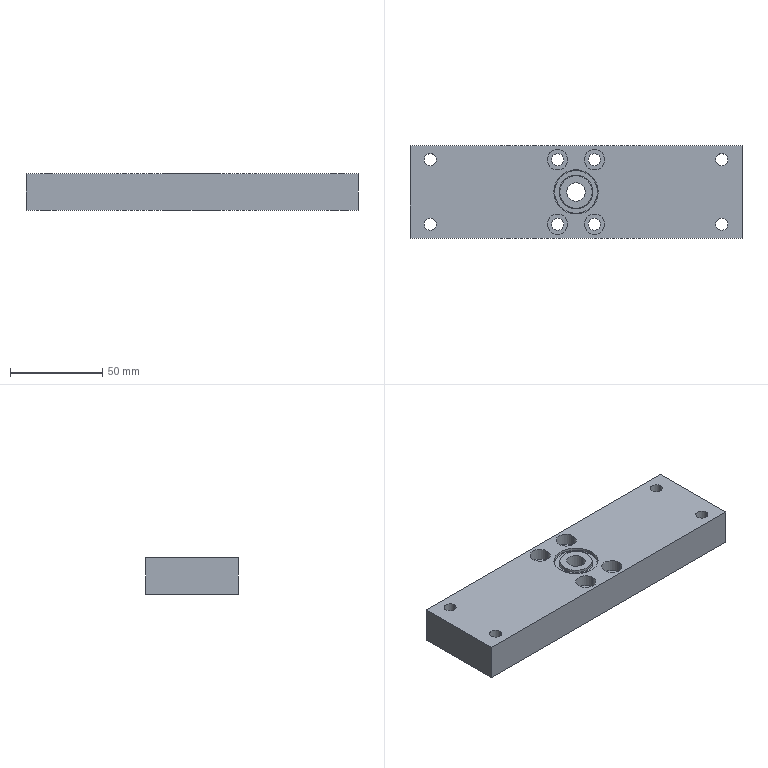Part | STEP file | M-05-116C_default | 1 solid | 68 faces | box 180 x 50 x 20 mm | volume 168438 mm3 | cylinder 42 | plane 18 | torus 8 | commonest cylinder face diameters 6.6 x16 11 x16 10 x2 17.6 x2 21.6 x2 24 x2